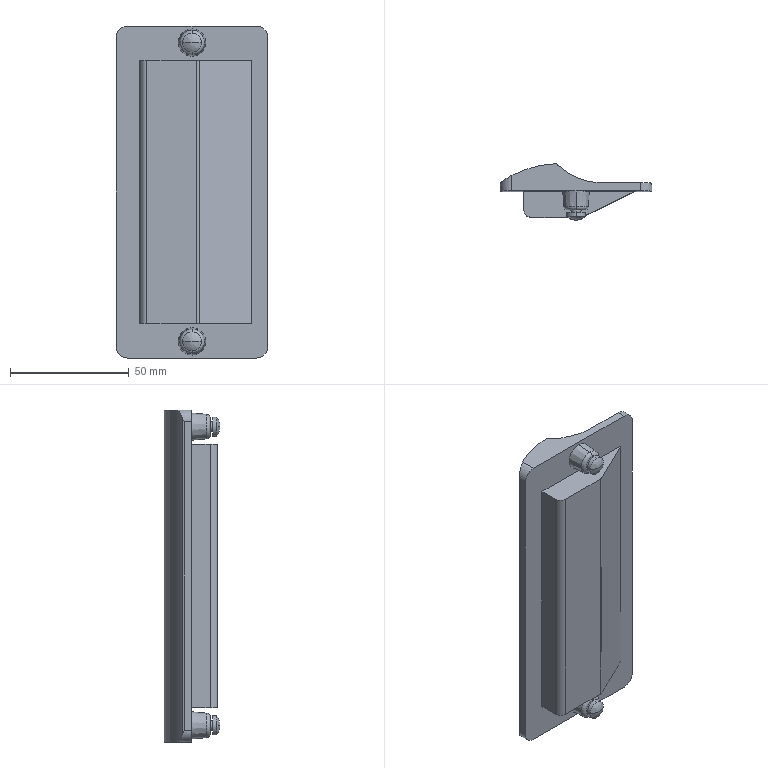Part | SolidWorks | features BaseBody 1 | 1 solid | 57 faces | box 64 x 23.592 x 140 mm | volume 48933 mm3 | cylinder 24 | plane 21 | spline 4 | cone 4 | torus 4 | commonest cylinder face diameters 2 x6 4 x4 8 x4 10 x4 52 x3 6 x2